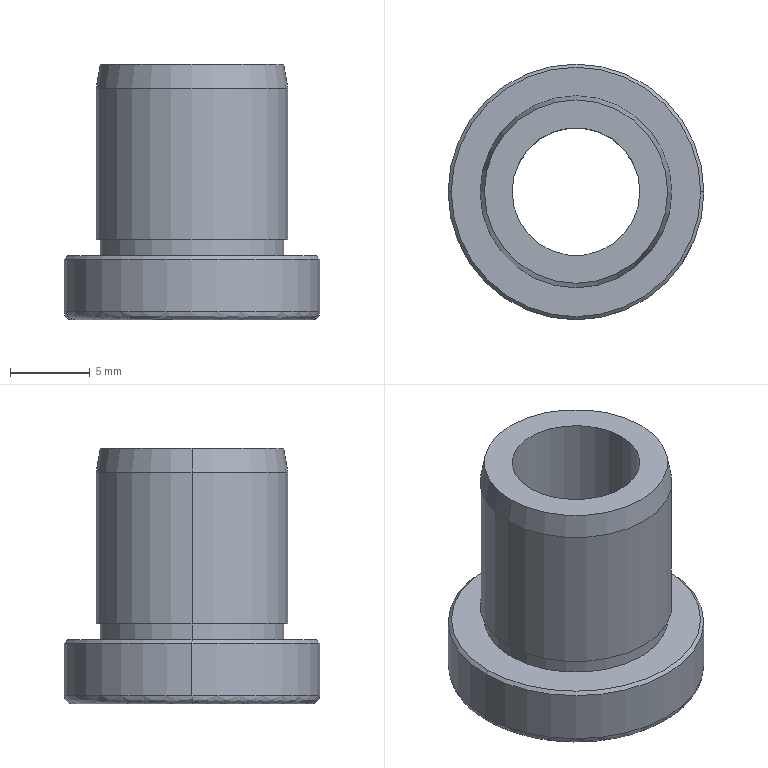Part | STEP file | Rotor step bushing JBH8-12 | 1 solid | 20 faces | box 16 x 16 x 16 mm | volume 1313 mm3 | cylinder 8 | spline 4 | cone 4 | plane 4 | commonest cylinder face diameters 8 x2 11.5 x2 12 x2 16 x2